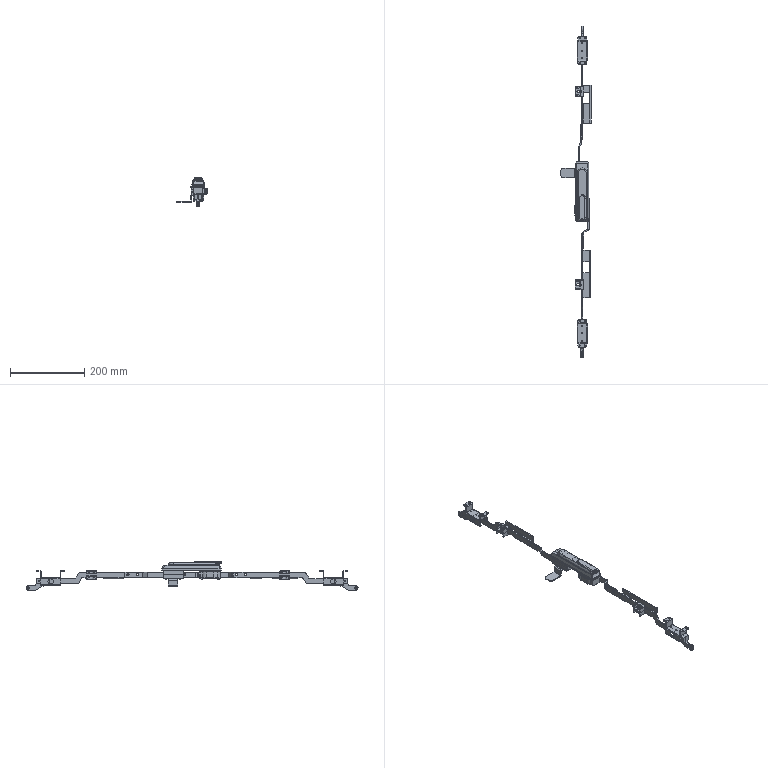Part | SolidWorks | 11 solids | 3520 faces | volume 240801 mm3 | plane 1909 | cylinder 1043 | spline 491 | cone 66 | torus 11 | commonest cylinder face diameters 1 x179 4.1 x102 4.8 x86 0.2 x61 2 x57 3 x51